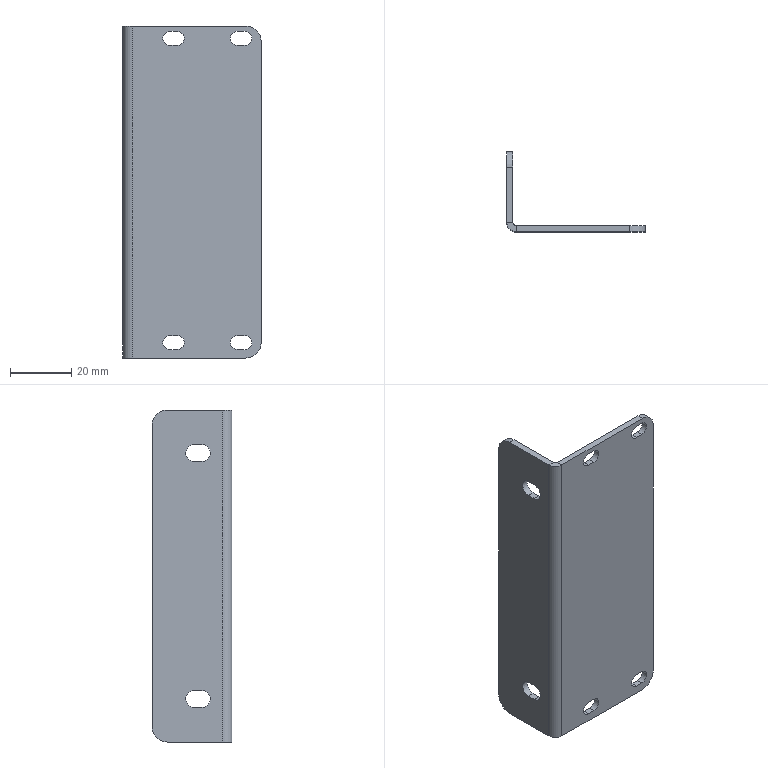Part | SolidWorks | features HoleWzd 2, Fillet 1, FlatPattern 1, SMBaseFlange 1, SheetMetal 1 | 1 solid | 42 faces | box 45 x 26 x 108 mm | volume 14308 mm3 | plane 24 | cylinder 18 | commonest cylinder face diameters 4.5 x8 5.5 x4 10 x4 2 x1 6 x1
STEP:
#1=CARTESIAN_POINT('',(0.,-23.,108.));
#2=VERTEX_POINT('',#1);
#3=CARTESIAN_POINT('',(2.,-23.,108.));
#4=VERTEX_POINT('',#3);
#5=CARTESIAN_POINT('',(0.,-23.,108.));
#6=DIRECTION('',(1.,0.,0.));
#7=VECTOR('',#6,1000.);
#8=LINE('',#5,#7);
#9=EDGE_CURVE('',#2,#4,#8,.T.);
#10=ORIENTED_EDGE('',*,*,#9,.F.);
#11=CARTESIAN_POINT('',(3.,-26.,108.));
#12=VERTEX_POINT('',#11);
#13=CARTESIAN_POINT('',(3.,-23.,108.));
#14=DIRECTION('',(0.,0.,1.));
#15=DIRECTION('',(-1.,0.,0.));
#16=AXIS2_PLACEMENT_3D('',#13,#14,#15);
#17=CIRCLE('',#16,3.);
#18=EDGE_CURVE('',#2,#12,#17,.T.);
#19=ORIENTED_EDGE('',*,*,#18,.T.);
#20=CARTESIAN_POINT('',(3.,-24.,108.));
#21=VERTEX_POINT('',#20);
#22=CARTESIAN_POINT('',(3.,-24.,108.));
#23=DIRECTION('',(0.,-1.,0.));
#24=VECTOR('',#23,1000.);
#25=LINE('',#22,#24);
#26=EDGE_CURVE('',#21,#12,#25,.T.);
#27=ORIENTED_EDGE('',*,*,#26,.F.);
#28=CARTESIAN_POINT('',(3.,-23.,108.));
#29=DIRECTION('',(0.,0.,1.));
#30=DIRECTION('',(1.,0.,0.));
#31=AXIS2_PLACEMENT_3D('',#28,#29,#30);
#32=CIRCLE('',#31,1.);
#33=EDGE_CURVE('',#4,#21,#32,.T.);
#34=ORIENTED_EDGE('',*,*,#33,.F.);
#35=EDGE_LOOP('',(#10,#19,#27,#34));
#36=FACE_OUTER_BOUND('',#35,.T.);
#37=CARTESIAN_POINT('',(0.,-23.,108.));
#38=DIRECTION('',(0.,0.,1.));
#39=DIRECTION('',(1.,0.,0.));
#40=AXIS2_PLACEMENT_3D('',#37,#38,#39);
#41=PLANE('',#40);
#42=ADVANCED_FACE('',(#36),#41,.T.);
#43=CARTESIAN_POINT('',(2.,-5.,108.));
#44=VERTEX_POINT('',#43);
#45=CARTESIAN_POINT('',(2.,0.,108.));
#46=DIRECTION('',(0.,-1.,0.));
#47=VECTOR('',#46,1000.);
#48=LINE('',#45,#47);
#49=EDGE_CURVE('',#44,#4,#48,.T.);
#50=ORIENTED_EDGE('',*,*,#49,.F.);
#51=CARTESIAN_POINT('',(0.,-5.,108.));
#52=VERTEX_POINT('',#51);
#53=CARTESIAN_POINT('',(3.,-5.,108.));
#54=DIRECTION('',(-1.,0.,0.));
#55=VECTOR('',#54,1000.);
#56=LINE('',#53,#55);
#57=EDGE_CURVE('',#44,#52,#56,.T.);
#58=ORIENTED_EDGE('',*,*,#57,.T.);
#59=CARTESIAN_POINT('',(0.,0.,108.));
#60=DIRECTION('',(0.,-1.,0.));
#61=VECTOR('',#60,1000.);
#62=LINE('',#59,#61);
#63=EDGE_CURVE('',#52,#2,#62,.T.);
#64=ORIENTED_EDGE('',*,*,#63,.T.);
#65=ORIENTED_EDGE('',*,*,#9,.T.);
#66=EDGE_LOOP('',(#50,#58,#64,#65));
#67=FACE_OUTER_BOUND('',#66,.T.);
#68=CARTESIAN_POINT('',(3.,-24.,108.));
#69=DIRECTION('',(0.,0.,1.));
#70=DIRECTION('',(1.,0.,0.));
#71=AXIS2_PLACEMENT_3D('',#68,#69,#70);
#72=PLANE('',#71);
#73=ADVANCED_FACE('',(#67),#72,.T.);
#74=CARTESIAN_POINT('',(3.,-26.,0.));
#75=VERTEX_POINT('',#74);
#76=CARTESIAN_POINT('',(3.,-24.,0.));
#77=VERTEX_POINT('',#76);
#78=CARTESIAN_POINT('',(3.,-26.,0.));
#79=DIRECTION('',(0.,1.,0.));
#80=VECTOR('',#79,1000.);
#81=LINE('',#78,#80);
#82=EDGE_CURVE('',#75,#77,#81,.T.);
#83=ORIENTED_EDGE('',*,*,#82,.F.);
#84=CARTESIAN_POINT('',(0.,-23.,0.));
#85=VERTEX_POINT('',#84);
#86=CARTESIAN_POINT('',(3.,-23.,0.));
#87=DIRECTION('',(0.,0.,1.));
#88=DIRECTION('',(-1.,0.,0.));
#89=AXIS2_PLACEMENT_3D('',#86,#87,#88);
#90=CIRCLE('',#89,3.);
#91=EDGE_CURVE('',#85,#75,#90,.T.);
#92=ORIENTED_EDGE('',*,*,#91,.F.);
#93=CARTESIAN_POINT('',(2.,-23.,0.));
#94=VERTEX_POINT('',#93);
#95=CARTESIAN_POINT('',(2.,-23.,0.));
#96=DIRECTION('',(-1.,0.,0.));
#97=VECTOR('',#96,1000.);
#98=LINE('',#95,#97);
#99=EDGE_CURVE('',#94,#85,#98,.T.);
#100=ORIENTED_EDGE('',*,*,#99,.F.);
#101=CARTESIAN_POINT('',(3.,-23.,0.));
#102=DIRECTION('',(0.,0.,1.));
#103=DIRECTION('',(1.,0.,0.));
#104=AXIS2_PLACEMENT_3D('',#101,#102,#103);
#105=CIRCLE('',#104,1.);
#106=EDGE_CURVE('',#94,#77,#105,.T.);
#107=ORIENTED_EDGE('',*,*,#106,.T.);
#108=EDGE_LOOP('',(#83,#92,#100,#107));
#109=FACE_OUTER_BOUND('',#108,.T.);
#110=CARTESIAN_POINT('',(3.,-26.,0.));
#111=DIRECTION('',(0.,0.,-1.));
#112=DIRECTION('',(-1.,0.,0.));
#113=AXIS2_PLACEMENT_3D('',#110,#111,#112);
#114=PLANE('',#113);
#115=ADVANCED_FACE('',(#109),#114,.T.);
#116=CARTESIAN_POINT('',(40.,-24.,0.));
#117=VERTEX_POINT('',#116);
#118=CARTESIAN_POINT('',(0.,-24.,0.));
#119=DIRECTION('',(1.,0.,0.));
#120=VECTOR('',#119,1000.);
#121=LINE('',#118,#120);
#122=EDGE_CURVE('',#77,#117,#121,.T.);
#123=ORIENTED_EDGE('',*,*,#122,.T.);
#124=CARTESIAN_POINT('',(40.,-26.,0.));
#125=VERTEX_POINT('',#124);
#126=CARTESIAN_POINT('',(40.,-23.,0.));
#127=DIRECTION('',(0.,-1.,0.));
#128=VECTOR('',#127,1000.);
#129=LINE('',#126,#128);
#130=EDGE_CURVE('',#117,#125,#129,.T.);
#131=ORIENTED_EDGE('',*,*,#130,.T.);
#132=CARTESIAN_POINT('',(0.,-26.,0.));
#133=DIRECTION('',(1.,0.,0.));
#134=VECTOR('',#133,1000.);
#135=LINE('',#132,#134);
#136=EDGE_CURVE('',#75,#125,#135,.T.);
#137=ORIENTED_EDGE('',*,*,#136,.F.);
#138=ORIENTED_EDGE('',*,*,#82,.T.);
#139=EDGE_LOOP('',(#123,#131,#137,#138));
#140=FACE_OUTER_BOUND('',#139,.T.);
#141=CARTESIAN_POINT('',(2.,-23.,0.));
#142=DIRECTION('',(0.,0.,-1.));
#143=DIRECTION('',(-1.,0.,0.));
#144=AXIS2_PLACEMENT_3D('',#141,#142,#143);
#145=PLANE('',#144);
#146=ADVANCED_FACE('',(#140),#145,.T.);
#147=CARTESIAN_POINT('',(37.25,-26.,7.25));
#148=VERTEX_POINT('',#147);
#149=CARTESIAN_POINT('',(39.75,-26.,7.25));
#150=VERTEX_POINT('',#149);
#151=CARTESIAN_POINT('',(0.,-26.,7.25));
#152=DIRECTION('',(1.,0.,0.));
#153=VECTOR('',#152,1000.);
#154=LINE('',#151,#153);
#155=EDGE_CURVE('',#148,#150,#154,.T.);
#156=ORIENTED_EDGE('',*,*,#155,.T.);
#157=CARTESIAN_POINT('',(39.75,-26.,2.75));
#158=VERTEX_POINT('',#157);
#159=CARTESIAN_POINT('',(39.75,-26.,5.));
#160=DIRECTION('',(0.,1.,0.));
#161=DIRECTION('',(0.,0.,1.));
#162=AXIS2_PLACEMENT_3D('',#159,#160,#161);
#163=CIRCLE('',#162,2.25);
#164=EDGE_CURVE('',#150,#158,#163,.T.);
#165=ORIENTED_EDGE('',*,*,#164,.T.);
#166=CARTESIAN_POINT('',(37.25,-26.,2.75));
#167=VERTEX_POINT('',#166);
#168=CARTESIAN_POINT('',(0.,-26.,2.75));
#169=DIRECTION('',(-1.,0.,0.));
#170=VECTOR('',#169,1000.);
#171=LINE('',#168,#170);
#172=EDGE_CURVE('',#158,#167,#171,.T.);
#173=ORIENTED_EDGE('',*,*,#172,.T.);
#174=CARTESIAN_POINT('',(37.25,-26.,5.));
#175=DIRECTION('',(0.,1.,0.));
#176=DIRECTION('',(0.,0.,1.));
#177=AXIS2_PLACEMENT_3D('',#174,#175,#176);
#178=CIRCLE('',#177,2.25);
#179=EDGE_CURVE('',#167,#148,#178,.T.);
#180=ORIENTED_EDGE('',*,*,#179,.T.);
#181=EDGE_LOOP('',(#156,#165,#173,#180));
#182=FACE_BOUND('',#181,.T.);
#183=CARTESIAN_POINT('',(17.75,-26.,7.25));
#184=VERTEX_POINT('',#183);
#185=CARTESIAN_POINT('',(17.75,-26.,2.75));
#186=VERTEX_POINT('',#185);
#187=CARTESIAN_POINT('',(17.75,-26.,5.));
#188=DIRECTION('',(0.,1.,0.));
#189=DIRECTION('',(0.,0.,1.));
#190=AXIS2_PLACEMENT_3D('',#187,#188,#189);
#191=CIRCLE('',#190,2.25);
#192=EDGE_CURVE('',#184,#186,#191,.T.);
#193=ORIENTED_EDGE('',*,*,#192,.T.);
#194=CARTESIAN_POINT('',(15.25,-26.,2.75));
#195=VERTEX_POINT('',#194);
#196=CARTESIAN_POINT('',(0.,-26.,2.75));
#197=DIRECTION('',(-1.,0.,0.));
#198=VECTOR('',#197,1000.);
#199=LINE('',#196,#198);
#200=EDGE_CURVE('',#186,#195,#199,.T.);
#201=ORIENTED_EDGE('',*,*,#200,.T.);
#202=CARTESIAN_POINT('',(15.25,-26.,7.25));
#203=VERTEX_POINT('',#202);
#204=CARTESIAN_POINT('',(15.25,-26.,5.));
#205=DIRECTION('',(0.,1.,0.));
#206=DIRECTION('',(0.,0.,1.));
#207=AXIS2_PLACEMENT_3D('',#204,#205,#206);
#208=CIRCLE('',#207,2.25);
#209=EDGE_CURVE('',#195,#203,#208,.T.);
#210=ORIENTED_EDGE('',*,*,#209,.T.);
#211=CARTESIAN_POINT('',(0.,-26.,7.25));
#212=DIRECTION('',(1.,0.,0.));
#213=VECTOR('',#212,1000.);
#214=LINE('',#211,#213);
#215=EDGE_CURVE('',#203,#184,#214,.T.);
#216=ORIENTED_EDGE('',*,*,#215,.T.);
#217=EDGE_LOOP('',(#193,#201,#210,#216));
#218=FACE_BOUND('',#217,.T.);
#219=CARTESIAN_POINT('',(39.75,-26.,101.75));
#220=VERTEX_POINT('',#219);
#221=CARTESIAN_POINT('',(37.25,-26.,101.75));
#222=VERTEX_POINT('',#221);
#223=CARTESIAN_POINT('',(0.,-26.,101.75));
#224=DIRECTION('',(-1.,0.,0.));
#225=VECTOR('',#224,1000.);
#226=LINE('',#223,#225);
#227=EDGE_CURVE('',#220,#222,#226,.T.);
#228=ORIENTED_EDGE('',*,*,#227,.T.);
#229=CARTESIAN_POINT('',(37.25,-26.,106.25));
#230=VERTEX_POINT('',#229);
#231=CARTESIAN_POINT('',(37.25,-26.,104.));
#232=DIRECTION('',(0.,1.,0.));
#233=DIRECTION('',(0.,0.,1.));
#234=AXIS2_PLACEMENT_3D('',#231,#232,#233);
#235=CIRCLE('',#234,2.25);
#236=EDGE_CURVE('',#222,#230,#235,.T.);
#237=ORIENTED_EDGE('',*,*,#236,.T.);
#238=CARTESIAN_POINT('',(39.75,-26.,106.25));
#239=VERTEX_POINT('',#238);
#240=CARTESIAN_POINT('',(0.,-26.,106.25));
#241=DIRECTION('',(1.,0.,0.));
#242=VECTOR('',#241,1000.);
#243=LINE('',#240,#242);
#244=EDGE_CURVE('',#230,#239,#243,.T.);
#245=ORIENTED_EDGE('',*,*,#244,.T.);
#246=CARTESIAN_POINT('',(39.75,-26.,104.));
#247=DIRECTION('',(0.,1.,0.));
#248=DIRECTION('',(0.,0.,1.));
#249=AXIS2_PLACEMENT_3D('',#246,#247,#248);
#250=CIRCLE('',#249,2.25);
#251=EDGE_CURVE('',#239,#220,#250,.T.);
#252=ORIENTED_EDGE('',*,*,#251,.T.);
#253=EDGE_LOOP('',(#228,#237,#245,#252));
#254=FACE_BOUND('',#253,.T.);
#255=CARTESIAN_POINT('',(17.75,-26.,106.25));
#256=VERTEX_POINT('',#255);
#257=CARTESIAN_POINT('',(17.75,-26.,101.75));
#258=VERTEX_POINT('',#257);
#259=CARTESIAN_POINT('',(17.75,-26.,104.));
#260=DIRECTION('',(0.,1.,0.));
#261=DIRECTION('',(0.,0.,1.));
#262=AXIS2_PLACEMENT_3D('',#259,#260,#261);
#263=CIRCLE('',#262,2.25);
#264=EDGE_CURVE('',#256,#258,#263,.T.);
#265=ORIENTED_EDGE('',*,*,#264,.T.);
#266=CARTESIAN_POINT('',(15.25,-26.,101.75));
#267=VERTEX_POINT('',#266);
#268=CARTESIAN_POINT('',(0.,-26.,101.75));
#269=DIRECTION('',(-1.,0.,0.));
#270=VECTOR('',#269,1000.);
#271=LINE('',#268,#270);
#272=EDGE_CURVE('',#258,#267,#271,.T.);
#273=ORIENTED_EDGE('',*,*,#272,.T.);
#274=CARTESIAN_POINT('',(15.25,-26.,106.25));
#275=VERTEX_POINT('',#274);
#276=CARTESIAN_POINT('',(15.25,-26.,104.));
#277=DIRECTION('',(0.,1.,0.));
#278=DIRECTION('',(0.,0.,1.));
#279=AXIS2_PLACEMENT_3D('',#276,#277,#278);
#280=CIRCLE('',#279,2.25);
#281=EDGE_CURVE('',#267,#275,#280,.T.);
#282=ORIENTED_EDGE('',*,*,#281,.T.);
#283=CARTESIAN_POINT('',(0.,-26.,106.25));
#284=DIRECTION('',(1.,0.,0.));
#285=VECTOR('',#284,1000.);
#286=LINE('',#283,#285);
#287=EDGE_CURVE('',#275,#256,#286,.T.);
#288=ORIENTED_EDGE('',*,*,#287,.T.);
#289=EDGE_LOOP('',(#265,#273,#282,#288));
#290=FACE_BOUND('',#289,.T.);
#291=ORIENTED_EDGE('',*,*,#136,.T.);
#292=CARTESIAN_POINT('',(45.,-26.,5.));
#293=VERTEX_POINT('',#292);
#294=CARTESIAN_POINT('',(40.,-26.,5.));
#295=DIRECTION('',(0.,-1.,0.));
#296=DIRECTION('',(0.,0.,1.));
#297=AXIS2_PLACEMENT_3D('',#294,#295,#296);
#298=CIRCLE('',#297,5.);
#299=EDGE_CURVE('',#125,#293,#298,.T.);
#300=ORIENTED_EDGE('',*,*,#299,.T.);
#301=CARTESIAN_POINT('',(45.,-26.,103.));
#302=VERTEX_POINT('',#301);
#303=CARTESIAN_POINT('',(45.,-26.,108.));
#304=DIRECTION('',(0.,0.,-1.));
#305=VECTOR('',#304,1000.);
#306=LINE('',#303,#305);
#307=EDGE_CURVE('',#302,#293,#306,.T.);
#308=ORIENTED_EDGE('',*,*,#307,.F.);
#309=CARTESIAN_POINT('',(40.,-26.,108.));
#310=VERTEX_POINT('',#309);
#311=CARTESIAN_POINT('',(40.,-26.,103.));
#312=DIRECTION('',(0.,-1.,0.));
#313=DIRECTION('',(0.,0.,1.));
#314=AXIS2_PLACEMENT_3D('',#311,#312,#313);
#315=CIRCLE('',#314,5.);
#316=EDGE_CURVE('',#302,#310,#315,.T.);
#317=ORIENTED_EDGE('',*,*,#316,.T.);
#318=CARTESIAN_POINT('',(0.,-26.,108.));
#319=DIRECTION('',(1.,0.,0.));
#320=VECTOR('',#319,1000.);
#321=LINE('',#318,#320);
#322=EDGE_CURVE('',#12,#310,#321,.T.);
#323=ORIENTED_EDGE('',*,*,#322,.F.);
#324=CARTESIAN_POINT('',(3.,-26.,108.));
#325=DIRECTION('',(0.,0.,-1.));
#326=VECTOR('',#325,1000.);
#327=LINE('',#324,#326);
#328=EDGE_CURVE('',#12,#75,#327,.T.);
#329=ORIENTED_EDGE('',*,*,#328,.T.);
#330=EDGE_LOOP('',(#291,#300,#308,#317,#323,#329));
#331=FACE_OUTER_BOUND('',#330,.T.);
#332=CARTESIAN_POINT('',(0.,-26.,108.));
#333=DIRECTION('',(0.,1.,0.));
#334=DIRECTION('',(0.,0.,1.));
#335=AXIS2_PLACEMENT_3D('',#332,#333,#334);
#336=PLANE('',#335);
#337=ADVANCED_FACE('',(#182,#218,#254,#290,#331),#336,.F.);
#338=ORIENTED_EDGE('',*,*,#307,.T.);
#339=CARTESIAN_POINT('',(45.,-24.,5.));
#340=VERTEX_POINT('',#339);
#341=CARTESIAN_POINT('',(45.,-24.,5.));
#342=DIRECTION('',(0.,1.,0.));
#343=VECTOR('',#342,1000.);
#344=LINE('',#341,#343);
#345=EDGE_CURVE('',#293,#340,#344,.T.);
#346=ORIENTED_EDGE('',*,*,#345,.T.);
#347=CARTESIAN_POINT('',(45.,-24.,103.));
#348=VERTEX_POINT('',#347);
#349=CARTESIAN_POINT('',(45.,-24.,108.));
#350=DIRECTION('',(0.,0.,-1.));
#351=VECTOR('',#350,1000.);
#352=LINE('',#349,#351);
#353=EDGE_CURVE('',#348,#340,#352,.T.);
#354=ORIENTED_EDGE('',*,*,#353,.F.);
#355=CARTESIAN_POINT('',(45.,-24.,103.));
#356=DIRECTION('',(0.,-1.,0.));
#357=VECTOR('',#356,1000.);
#358=LINE('',#355,#357);
#359=EDGE_CURVE('',#348,#302,#358,.T.);
#360=ORIENTED_EDGE('',*,*,#359,.T.);
#361=EDGE_LOOP('',(#338,#346,#354,#360));
#362=FACE_OUTER_BOUND('',#361,.T.);
#363=CARTESIAN_POINT('',(45.,-24.,108.));
#364=DIRECTION('',(1.,0.,0.));
#365=DIRECTION('',(0.,0.,-1.));
#366=AXIS2_PLACEMENT_3D('',#363,#364,#365);
#367=PLANE('',#366);
#368=ADVANCED_FACE('',(#362),#367,.T.);
#369=CARTESIAN_POINT('',(37.25,-24.,7.25));
#370=VERTEX_POINT('',#369);
#371=CARTESIAN_POINT('',(39.75,-24.,7.25));
#372=VERTEX_POINT('',#371);
#373=CARTESIAN_POINT('',(37.25,-24.,7.25));
#374=DIRECTION('',(1.,0.,0.));
#375=VECTOR('',#374,1000.);
#376=LINE('',#373,#375);
#377=EDGE_CURVE('',#370,#372,#376,.T.);
#378=ORIENTED_EDGE('',*,*,#377,.F.);
#379=CARTESIAN_POINT('',(37.25,-24.,2.75));
#380=VERTEX_POINT('',#379);
#381=CARTESIAN_POINT('',(37.25,-24.,5.));
#382=DIRECTION('',(0.,1.,0.));
#383=DIRECTION('',(0.,0.,1.));
#384=AXIS2_PLACEMENT_3D('',#381,#382,#383);
#385=CIRCLE('',#384,2.25);
#386=EDGE_CURVE('',#380,#370,#385,.T.);
#387=ORIENTED_EDGE('',*,*,#386,.F.);
#388=CARTESIAN_POINT('',(39.75,-24.,2.75));
#389=VERTEX_POINT('',#388);
#390=CARTESIAN_POINT('',(37.25,-24.,2.75));
#391=DIRECTION('',(1.,0.,0.));
#392=VECTOR('',#391,1000.);
#393=LINE('',#390,#392);
#394=EDGE_CURVE('',#380,#389,#393,.T.);
#395=ORIENTED_EDGE('',*,*,#394,.T.);
#396=CARTESIAN_POINT('',(39.75,-24.,5.));
#397=DIRECTION('',(0.,1.,0.));
#398=DIRECTION('',(0.,0.,1.));
#399=AXIS2_PLACEMENT_3D('',#396,#397,#398);
#400=CIRCLE('',#399,2.25);
#401=EDGE_CURVE('',#372,#389,#400,.T.);
#402=ORIENTED_EDGE('',*,*,#401,.F.);
#403=EDGE_LOOP('',(#378,#387,#395,#402));
#404=FACE_BOUND('',#403,.T.);
#405=CARTESIAN_POINT('',(15.25,-24.,7.25));
#406=VERTEX_POINT('',#405);
#407=CARTESIAN_POINT('',(17.75,-24.,7.25));
#408=VERTEX_POINT('',#407);
#409=CARTESIAN_POINT('',(15.25,-24.,7.25));
#410=DIRECTION('',(1.,0.,0.));
#411=VECTOR('',#410,1000.);
#412=LINE('',#409,#411);
#413=EDGE_CURVE('',#406,#408,#412,.T.);
#414=ORIENTED_EDGE('',*,*,#413,.F.);
#415=CARTESIAN_POINT('',(15.25,-24.,2.75));
#416=VERTEX_POINT('',#415);
#417=CARTESIAN_POINT('',(15.25,-24.,5.));
#418=DIRECTION('',(0.,1.,0.));
#419=DIRECTION('',(0.,0.,1.));
#420=AXIS2_PLACEMENT_3D('',#417,#418,#419);
#421=CIRCLE('',#420,2.25);
#422=EDGE_CURVE('',#416,#406,#421,.T.);
#423=ORIENTED_EDGE('',*,*,#422,.F.);
#424=CARTESIAN_POINT('',(17.75,-24.,2.75));
#425=VERTEX_POINT('',#424);
#426=CARTESIAN_POINT('',(15.25,-24.,2.75));
#427=DIRECTION('',(1.,0.,0.));
#428=VECTOR('',#427,1000.);
#429=LINE('',#426,#428);
#430=EDGE_CURVE('',#416,#425,#429,.T.);
#431=ORIENTED_EDGE('',*,*,#430,.T.);
#432=CARTESIAN_POINT('',(17.75,-24.,5.));
#433=DIRECTION('',(0.,1.,0.));
#434=DIRECTION('',(0.,0.,1.));
#435=AXIS2_PLACEMENT_3D('',#432,#433,#434);
#436=CIRCLE('',#435,2.25);
#437=EDGE_CURVE('',#408,#425,#436,.T.);
#438=ORIENTED_EDGE('',*,*,#437,.F.);
#439=EDGE_LOOP('',(#414,#423,#431,#438));
#440=FACE_BOUND('',#439,.T.);
#441=CARTESIAN_POINT('',(39.75,-24.,106.25));
#442=VERTEX_POINT('',#441);
#443=CARTESIAN_POINT('',(39.75,-24.,101.75));
#444=VERTEX_POINT('',#443);
#445=CARTESIAN_POINT('',(39.75,-24.,104.));
#446=DIRECTION('',(0.,1.,0.));
#447=DIRECTION('',(0.,0.,1.));
#448=AXIS2_PLACEMENT_3D('',#445,#446,#447);
#449=CIRCLE('',#448,2.25);
#450=EDGE_CURVE('',#442,#444,#449,.T.);
#451=ORIENTED_EDGE('',*,*,#450,.F.);
#452=CARTESIAN_POINT('',(37.25,-24.,106.25));
#453=VERTEX_POINT('',#452);
#454=CARTESIAN_POINT('',(37.25,-24.,106.25));
#455=DIRECTION('',(1.,0.,0.));
#456=VECTOR('',#455,1000.);
#457=LINE('',#454,#456);
#458=EDGE_CURVE('',#453,#442,#457,.T.);
#459=ORIENTED_EDGE('',*,*,#458,.F.);
#460=CARTESIAN_POINT('',(37.25,-24.,101.75));
#461=VERTEX_POINT('',#460);
#462=CARTESIAN_POINT('',(37.25,-24.,104.));
#463=DIRECTION('',(0.,1.,0.));
#464=DIRECTION('',(0.,0.,1.));
#465=AXIS2_PLACEMENT_3D('',#462,#463,#464);
#466=CIRCLE('',#465,2.25);
#467=EDGE_CURVE('',#461,#453,#466,.T.);
#468=ORIENTED_EDGE('',*,*,#467,.F.);
#469=CARTESIAN_POINT('',(37.25,-24.,101.75));
#470=DIRECTION('',(1.,0.,0.));
#471=VECTOR('',#470,1000.);
#472=LINE('',#469,#471);
#473=EDGE_CURVE('',#461,#444,#472,.T.);
#474=ORIENTED_EDGE('',*,*,#473,.T.);
#475=EDGE_LOOP('',(#451,#459,#468,#474));
#476=FACE_BOUND('',#475,.T.);
#477=CARTESIAN_POINT('',(15.25,-24.,106.25));
#478=VERTEX_POINT('',#477);
#479=CARTESIAN_POINT('',(17.75,-24.,106.25));
#480=VERTEX_POINT('',#479);
#481=CARTESIAN_POINT('',(15.25,-24.,106.25));
#482=DIRECTION('',(1.,0.,0.));
#483=VECTOR('',#482,1000.);
#484=LINE('',#481,#483);
#485=EDGE_CURVE('',#478,#480,#484,.T.);
#486=ORIENTED_EDGE('',*,*,#485,.F.);
#487=CARTESIAN_POINT('',(15.25,-24.,101.75));
#488=VERTEX_POINT('',#487);
#489=CARTESIAN_POINT('',(15.25,-24.,104.));
#490=DIRECTION('',(0.,1.,0.));
#491=DIRECTION('',(0.,0.,1.));
#492=AXIS2_PLACEMENT_3D('',#489,#490,#491);
#493=CIRCLE('',#492,2.25);
#494=EDGE_CURVE('',#488,#478,#493,.T.);
#495=ORIENTED_EDGE('',*,*,#494,.F.);
#496=CARTESIAN_POINT('',(17.75,-24.,101.75));
#497=VERTEX_POINT('',#496);
#498=CARTESIAN_POINT('',(15.25,-24.,101.75));
#499=DIRECTION('',(1.,0.,0.));
#500=VECTOR('',#499,1000.);
#501=LINE('',#498,#500);
#502=EDGE_CURVE('',#488,#497,#501,.T.);
#503=ORIENTED_EDGE('',*,*,#502,.T.);
#504=CARTESIAN_POINT('',(17.75,-24.,104.));
#505=DIRECTION('',(0.,1.,0.));
#506=DIRECTION('',(0.,0.,1.));
#507=AXIS2_PLACEMENT_3D('',#504,#505,#506);
#508=CIRCLE('',#507,2.25);
#509=EDGE_CURVE('',#480,#497,#508,.T.);
#510=ORIENTED_EDGE('',*,*,#509,.F.);
#511=EDGE_LOOP('',(#486,#495,#503,#510));
#512=FACE_BOUND('',#511,.T.);
#513=ORIENTED_EDGE('',*,*,#353,.T.);
#514=CARTESIAN_POINT('',(40.,-24.,5.));
#515=DIRECTION('',(0.,1.,0.));
#516=DIRECTION('',(0.,0.,1.));
#517=AXIS2_PLACEMENT_3D('',#514,#515,#516);
#518=CIRCLE('',#517,5.);
#519=EDGE_CURVE('',#340,#117,#518,.T.);
#520=ORIENTED_EDGE('',*,*,#519,.T.);
#521=ORIENTED_EDGE('',*,*,#122,.F.);
#522=CARTESIAN_POINT('',(3.,-24.,108.));
#523=DIRECTION('',(0.,0.,-1.));
#524=VECTOR('',#523,1000.);
#525=LINE('',#522,#524);
#526=EDGE_CURVE('',#21,#77,#525,.T.);
#527=ORIENTED_EDGE('',*,*,#526,.F.);
#528=CARTESIAN_POINT('',(40.,-24.,108.));
#529=VERTEX_POINT('',#528);
#530=CARTESIAN_POINT('',(0.,-24.,108.));
#531=DIRECTION('',(1.,0.,0.));
#532=VECTOR('',#531,1000.);
#533=LINE('',#530,#532);
#534=EDGE_CURVE('',#21,#529,#533,.T.);
#535=ORIENTED_EDGE('',*,*,#534,.T.);
#536=CARTESIAN_POINT('',(40.,-24.,103.));
#537=DIRECTION('',(0.,1.,0.));
#538=DIRECTION('',(0.,0.,1.));
#539=AXIS2_PLACEMENT_3D('',#536,#537,#538);
#540=CIRCLE('',#539,5.);
#541=EDGE_CURVE('',#529,#348,#540,.T.);
#542=ORIENTED_EDGE('',*,*,#541,.T.);
#543=EDGE_LOOP('',(#513,#520,#521,#527,#535,#542));
#544=FACE_OUTER_BOUND('',#543,.T.);
#545=CARTESIAN_POINT('',(0.,-24.,108.));
#546=DIRECTION('',(0.,1.,0.));
#547=DIRECTION('',(0.,0.,1.));
#548=AXIS2_PLACEMENT_3D('',#545,#546,#547);
#549=PLANE('',#548);
#550=ADVANCED_FACE('',(#404,#440,#476,#512,#544),#549,.T.);
#551=ORIENTED_EDGE('',*,*,#106,.F.);
#552=CARTESIAN_POINT('',(2.,-23.,108.));
#553=DIRECTION('',(0.,0.,-1.));
#554=VECTOR('',#553,1000.);
#555=LINE('',#552,#554);
#556=EDGE_CURVE('',#4,#94,#555,.T.);
#557=ORIENTED_EDGE('',*,*,#556,.F.);
#558=ORIENTED_EDGE('',*,*,#33,.T.);
#559=ORIENTED_EDGE('',*,*,#526,.T.);
#560=EDGE_LOOP('',(#551,#557,#558,#559));
#561=FACE_OUTER_BOUND('',#560,.T.);
#562=CARTESIAN_POINT('',(3.,-23.,108.));
#563=DIRECTION('',(0.,0.,-1.));
#564=DIRECTION('',(-1.,0.,0.));
#565=AXIS2_PLACEMENT_3D('',#562,#563,#564);
#566=CYLINDRICAL_SURFACE('',#565,1.);
#567=ADVANCED_FACE('',(#561),#566,.F.);
#568=CARTESIAN_POINT('',(2.,-13.75,11.25));
#569=VERTEX_POINT('',#568);
#570=CARTESIAN_POINT('',(2.,-13.75,16.75));
#571=VERTEX_POINT('',#570);
#572=CARTESIAN_POINT('',(2.,-13.75,14.));
#573=DIRECTION('',(1.,0.,0.));
#574=DIRECTION('',(0.,0.,-1.));
#575=AXIS2_PLACEMENT_3D('',#572,#573,#574);
#576=CIRCLE('',#575,2.75);
#577=EDGE_CURVE('',#569,#571,#576,.T.);
#578=ORIENTED_EDGE('',*,*,#577,.F.);
#579=CARTESIAN_POINT('',(2.,-16.25,11.25));
#580=VERTEX_POINT('',#579);
#581=CARTESIAN_POINT('',(2.,-16.25,11.25));
#582=DIRECTION('',(0.,1.,0.));
#583=VECTOR('',#582,1000.);
#584=LINE('',#581,#583);
#585=EDGE_CURVE('',#580,#569,#584,.T.);
#586=ORIENTED_EDGE('',*,*,#585,.F.);
#587=CARTESIAN_POINT('',(2.,-16.25,16.75));
#588=VERTEX_POINT('',#587);
#589=CARTESIAN_POINT('',(2.,-16.25,14.));
#590=DIRECTION('',(1.,0.,0.));
#591=DIRECTION('',(0.,0.,-1.));
#592=AXIS2_PLACEMENT_3D('',#589,#590,#591);
#593=CIRCLE('',#592,2.75);
#594=EDGE_CURVE('',#588,#580,#593,.T.);
#595=ORIENTED_EDGE('',*,*,#594,.F.);
#596=CARTESIAN_POINT('',(2.,-16.25,16.75));
#597=DIRECTION('',(0.,1.,0.));
#598=VECTOR('',#597,1000.);
#599=LINE('',#596,#598);
#600=EDGE_CURVE('',#588,#571,#599,.T.);
#601=ORIENTED_EDGE('',*,*,#600,.T.);
#602=EDGE_LOOP('',(#578,#586,#595,#601));
#603=FACE_BOUND('',#602,.T.);
#604=CARTESIAN_POINT('',(2.,-13.75,91.25));
#605=VERTEX_POINT('',#604);
#606=CARTESIAN_POINT('',(2.,-13.75,96.75));
#607=VERTEX_POINT('',#606);
#608=CARTESIAN_POINT('',(2.,-13.75,94.));
#609=DIRECTION('',(1.,0.,0.));
#610=DIRECTION('',(0.,0.,-1.));
#611=AXIS2_PLACEMENT_3D('',#608,#609,#610);
#612=CIRCLE('',#611,2.75);
#613=EDGE_CURVE('',#605,#607,#612,.T.);
#614=ORIENTED_EDGE('',*,*,#613,.F.);
#615=CARTESIAN_POINT('',(2.,-16.25,91.25));
#616=VERTEX_POINT('',#615);
#617=CARTESIAN_POINT('',(2.,-16.25,91.25));
#618=DIRECTION('',(0.,1.,0.));
#619=VECTOR('',#618,1000.);
#620=LINE('',#617,#619);
#621=EDGE_CURVE('',#616,#605,#620,.T.);
#622=ORIENTED_EDGE('',*,*,#621,.F.);
#623=CARTESIAN_POINT('',(2.,-16.25,96.75));
#624=VERTEX_POINT('',#623);
#625=CARTESIAN_POINT('',(2.,-16.25,94.));
#626=DIRECTION('',(1.,0.,0.));
#627=DIRECTION('',(0.,0.,-1.));
#628=AXIS2_PLACEMENT_3D('',#625,#626,#627);
#629=CIRCLE('',#628,2.75);
#630=EDGE_CURVE('',#624,#616,#629,.T.);
#631=ORIENTED_EDGE('',*,*,#630,.F.);
#632=CARTESIAN_POINT('',(2.,-16.25,96.75));
#633=DIRECTION('',(0.,1.,0.));
#634=VECTOR('',#633,1000.);
#635=LINE('',#632,#634);
#636=EDGE_CURVE('',#624,#607,#635,.T.);
#637=ORIENTED_EDGE('',*,*,#636,.T.);
#638=EDGE_LOOP('',(#614,#622,#631,#637));
#639=FACE_BOUND('',#638,.T.);
#640=CARTESIAN_POINT('',(2.,0.,103.));
#641=VERTEX_POINT('',#640);
#642=CARTESIAN_POINT('',(2.,0.,5.));
#643=VERTEX_POINT('',#642);
#644=CARTESIAN_POINT('',(2.,0.,108.));
#645=DIRECTION('',(0.,0.,-1.));
#646=VECTOR('',#645,1000.);
#647=LINE('',#644,#646);
#648=EDGE_CURVE('',#641,#643,#647,.T.);
#649=ORIENTED_EDGE('',*,*,#648,.F.);
#650=CARTESIAN_POINT('',(2.,-5.,103.));
#651=DIRECTION('',(1.,0.,0.));
#652=DIRECTION('',(0.,1.,0.));
#653=AXIS2_PLACEMENT_3D('',#650,#651,#652);
#654=CIRCLE('',#653,5.);
#655=EDGE_CURVE('',#641,#44,#654,.T.);
#656=ORIENTED_EDGE('',*,*,#655,.T.);
#657=ORIENTED_EDGE('',*,*,#49,.T.);
#658=ORIENTED_EDGE('',*,*,#556,.T.);
#659=CARTESIAN_POINT('',(2.,-5.,0.));
#660=VERTEX_POINT('',#659);
#661=CARTESIAN_POINT('',(2.,0.,0.));
#662=DIRECTION('',(0.,-1.,0.));
#663=VECTOR('',#662,1000.);
#664=LINE('',#661,#663);
#665=EDGE_CURVE('',#660,#94,#664,.T.);
#666=ORIENTED_EDGE('',*,*,#665,.F.);
#667=CARTESIAN_POINT('',(2.,-5.,5.));
#668=DIRECTION('',(1.,0.,0.));
#669=DIRECTION('',(0.,1.,0.));
#670=AXIS2_PLACEMENT_3D('',#667,#668,#669);
#671=CIRCLE('',#670,5.);
#672=EDGE_CURVE('',#660,#643,#671,.T.);
#673=ORIENTED_EDGE('',*,*,#672,.T.);
#674=EDGE_LOOP('',(#649,#656,#657,#658,#666,#673));
#675=FACE_OUTER_BOUND('',#674,.T.);
#676=CARTESIAN_POINT('',(2.,0.,108.));
#677=DIRECTION('',(1.,0.,0.));
#678=DIRECTION('',(0.,1.,0.));
#679=AXIS2_PLACEMENT_3D('',#676,#677,#678);
#680=PLANE('',#679);
#681=ADVANCED_FACE('',(#603,#639,#675),#680,.T.);
#682=CARTESIAN_POINT('',(0.,0.,103.));
#683=VERTEX_POINT('',#682);
#684=CARTESIAN_POINT('',(0.,0.,5.));
#685=VERTEX_POINT('',#684);
#686=CARTESIAN_POINT('',(0.,0.,108.));
#687=DIRECTION('',(0.,0.,-1.));
#688=VECTOR('',#687,1000.);
#689=LINE('',#686,#688);
#690=EDGE_CURVE('',#683,#685,#689,.T.);
#691=ORIENTED_EDGE('',*,*,#690,.F.);
#692=CARTESIAN_POINT('',(0.,0.,103.));
#693=DIRECTION('',(1.,0.,0.));
#694=VECTOR('',#693,1000.);
#695=LINE('',#692,#694);
#696=EDGE_CURVE('',#683,#641,#695,.T.);
#697=ORIENTED_EDGE('',*,*,#696,.T.);
#698=ORIENTED_EDGE('',*,*,#648,.T.);
#699=CARTESIAN_POINT('',(0.,0.,5.));
#700=DIRECTION('',(-1.,0.,0.));
#701=VECTOR('',#700,1000.);
#702=LINE('',#699,#701);
#703=EDGE_CURVE('',#643,#685,#702,.T.);
#704=ORIENTED_EDGE('',*,*,#703,.T.);
#705=EDGE_LOOP('',(#691,#697,#698,#704));
#706=FACE_OUTER_BOUND('',#705,.T.);
#707=CARTESIAN_POINT('',(0.,0.,108.));
#708=DIRECTION('',(0.,1.,0.));
#709=DIRECTION('',(-1.,0.,0.));
#710=AXIS2_PLACEMENT_3D('',#707,#708,#709);
#711=PLANE('',#710);
#712=ADVANCED_FACE('',(#706),#711,.T.);
#713=CARTESIAN_POINT('',(0.,-13.75,16.75));
#714=VERTEX_POINT('',#713);
#715=CARTESIAN_POINT('',(0.,-16.25,16.75));
#716=VERTEX_POINT('',#715);
#717=CARTESIAN_POINT('',(0.,0.,16.75));
#718=DIRECTION('',(0.,-1.,0.));
#719=VECTOR('',#718,1000.);
#720=LINE('',#717,#719);
#721=EDGE_CURVE('',#714,#716,#720,.T.);
#722=ORIENTED_EDGE('',*,*,#721,.T.);
#723=CARTESIAN_POINT('',(0.,-16.25,11.25));
#724=VERTEX_POINT('',#723);
#725=CARTESIAN_POINT('',(0.,-16.25,14.));
#726=DIRECTION('',(1.,0.,0.));
#727=DIRECTION('',(0.,1.,0.));
#728=AXIS2_PLACEMENT_3D('',#725,#726,#727);
#729=CIRCLE('',#728,2.75);
#730=EDGE_CURVE('',#716,#724,#729,.T.);
#731=ORIENTED_EDGE('',*,*,#730,.T.);
#732=CARTESIAN_POINT('',(0.,-13.75,11.25));
#733=VERTEX_POINT('',#732);
#734=CARTESIAN_POINT('',(0.,0.,11.25));
#735=DIRECTION('',(0.,1.,0.));
#736=VECTOR('',#735,1000.);
#737=LINE('',#734,#736);
#738=EDGE_CURVE('',#724,#733,#737,.T.);
#739=ORIENTED_EDGE('',*,*,#738,.T.);
#740=CARTESIAN_POINT('',(0.,-13.75,14.));
#741=DIRECTION('',(1.,0.,0.));
#742=DIRECTION('',(0.,1.,0.));
#743=AXIS2_PLACEMENT_3D('',#740,#741,#742);
#744=CIRCLE('',#743,2.75);
#745=EDGE_CURVE('',#733,#714,#744,.T.);
#746=ORIENTED_EDGE('',*,*,#745,.T.);
#747=EDGE_LOOP('',(#722,#731,#739,#746));
#748=FACE_BOUND('',#747,.T.);
#749=CARTESIAN_POINT('',(0.,-13.75,96.75));
#750=VERTEX_POINT('',#749);
#751=CARTESIAN_POINT('',(0.,-16.25,96.75));
#752=VERTEX_POINT('',#751);
#753=CARTESIAN_POINT('',(0.,0.,96.75));
#754=DIRECTION('',(0.,-1.,0.));
#755=VECTOR('',#754,1000.);
#756=LINE('',#753,#755);
#757=EDGE_CURVE('',#750,#752,#756,.T.);
#758=ORIENTED_EDGE('',*,*,#757,.T.);
#759=CARTESIAN_POINT('',(0.,-16.25,91.25));
#760=VERTEX_POINT('',#759);
#761=CARTESIAN_POINT('',(0.,-16.25,94.));
#762=DIRECTION('',(1.,0.,0.));
#763=DIRECTION('',(0.,1.,0.));
#764=AXIS2_PLACEMENT_3D('',#761,#762,#763);
#765=CIRCLE('',#764,2.75);
#766=EDGE_CURVE('',#752,#760,#765,.T.);
#767=ORIENTED_EDGE('',*,*,#766,.T.);
#768=CARTESIAN_POINT('',(0.,-13.75,91.25));
#769=VERTEX_POINT('',#768);
#770=CARTESIAN_POINT('',(0.,0.,91.25));
#771=DIRECTION('',(0.,1.,0.));
#772=VECTOR('',#771,1000.);
#773=LINE('',#770,#772);
#774=EDGE_CURVE('',#760,#769,#773,.T.);
#775=ORIENTED_EDGE('',*,*,#774,.T.);
#776=CARTESIAN_POINT('',(0.,-13.75,94.));
#777=DIRECTION('',(1.,0.,0.));
#778=DIRECTION('',(0.,1.,0.));
#779=AXIS2_PLACEMENT_3D('',#776,#777,#778);
#780=CIRCLE('',#779,2.75);
#781=EDGE_CURVE('',#769,#750,#780,.T.);
#782=ORIENTED_EDGE('',*,*,#781,.T.);
#783=EDGE_LOOP('',(#758,#767,#775,#782));
#784=FACE_BOUND('',#783,.T.);
#785=ORIENTED_EDGE('',*,*,#63,.F.);
#786=CARTESIAN_POINT('',(0.,-5.,103.));
#787=DIRECTION('',(-1.,0.,0.));
#788=DIRECTION('',(0.,1.,0.));
#789=AXIS2_PLACEMENT_3D('',#786,#787,#788);
#790=CIRCLE('',#789,5.);
#791=EDGE_CURVE('',#52,#683,#790,.T.);
#792=ORIENTED_EDGE('',*,*,#791,.T.);
#793=ORIENTED_EDGE('',*,*,#690,.T.);
#794=CARTESIAN_POINT('',(0.,-5.,0.));
#795=VERTEX_POINT('',#794);
#796=CARTESIAN_POINT('',(0.,-5.,5.));
#797=DIRECTION('',(-1.,0.,0.));
#798=DIRECTION('',(0.,1.,0.));
#799=AXIS2_PLACEMENT_3D('',#796,#797,#798);
#800=CIRCLE('',#799,5.);
#801=EDGE_CURVE('',#685,#795,#800,.T.);
#802=ORIENTED_EDGE('',*,*,#801,.T.);
#803=CARTESIAN_POINT('',(0.,0.,0.));
#804=DIRECTION('',(0.,-1.,0.));
#805=VECTOR('',#804,1000.);
#806=LINE('',#803,#805);
#807=EDGE_CURVE('',#795,#85,#806,.T.);
#808=ORIENTED_EDGE('',*,*,#807,.T.);
#809=CARTESIAN_POINT('',(0.,-23.,108.));
#810=DIRECTION('',(0.,0.,-1.));
#811=VECTOR('',#810,1000.);
#812=LINE('',#809,#811);
#813=EDGE_CURVE('',#2,#85,#812,.T.);
#814=ORIENTED_EDGE('',*,*,#813,.F.);
#815=EDGE_LOOP('',(#785,#792,#793,#802,#808,#814));
#816=FACE_OUTER_BOUND('',#815,.T.);
#817=CARTESIAN_POINT('',(0.,0.,108.));
#818=DIRECTION('',(1.,0.,0.));
#819=DIRECTION('',(0.,1.,0.));
#820=AXIS2_PLACEMENT_3D('',#817,#818,#819);
#821=PLANE('',#820);
#822=ADVANCED_FACE('',(#748,#784,#816),#821,.F.);
#823=ORIENTED_EDGE('',*,*,#91,.T.);
#824=ORIENTED_EDGE('',*,*,#328,.F.);
#825=ORIENTED_EDGE('',*,*,#18,.F.);
#826=ORIENTED_EDGE('',*,*,#813,.T.);
#827=EDGE_LOOP('',(#823,#824,#825,#826));
#828=FACE_OUTER_BOUND('',#827,.T.);
#829=CARTESIAN_POINT('',(3.,-23.,108.));
#830=DIRECTION('',(0.,0.,-1.));
#831=DIRECTION('',(-1.,0.,0.));
#832=AXIS2_PLACEMENT_3D('',#829,#830,#831);
#833=CYLINDRICAL_SURFACE('',#832,3.);
#834=ADVANCED_FACE('',(#828),#833,.T.);
#835=ORIENTED_EDGE('',*,*,#322,.T.);
#836=CARTESIAN_POINT('',(40.,-23.,108.));
#837=DIRECTION('',(0.,1.,0.));
#838=VECTOR('',#837,1000.);
#839=LINE('',#836,#838);
#840=EDGE_CURVE('',#310,#529,#839,.T.);
#841=ORIENTED_EDGE('',*,*,#840,.T.);
#842=ORIENTED_EDGE('',*,*,#534,.F.);
#843=ORIENTED_EDGE('',*,*,#26,.T.);
#844=EDGE_LOOP('',(#835,#841,#842,#843));
#845=FACE_OUTER_BOUND('',#844,.T.);
#846=CARTESIAN_POINT('',(3.,-23.,108.));
#847=DIRECTION('',(0.,0.,1.));
#848=DIRECTION('',(1.,0.,0.));
#849=AXIS2_PLACEMENT_3D('',#846,#847,#848);
#850=PLANE('',#849);
#851=ADVANCED_FACE('',(#845),#850,.T.);
#852=ORIENTED_EDGE('',*,*,#807,.F.);
#853=CARTESIAN_POINT('',(2.,-5.,0.));
#854=DIRECTION('',(1.,0.,0.));
#855=VECTOR('',#854,1000.);
#856=LINE('',#853,#855);
#857=EDGE_CURVE('',#795,#660,#856,.T.);
#858=ORIENTED_EDGE('',*,*,#857,.T.);
#859=ORIENTED_EDGE('',*,*,#665,.T.);
#860=ORIENTED_EDGE('',*,*,#99,.T.);
#861=EDGE_LOOP('',(#852,#858,#859,#860));
#862=FACE_OUTER_BOUND('',#861,.T.);
#863=CARTESIAN_POINT('',(3.,-23.,0.));
#864=DIRECTION('',(0.,0.,1.));
#865=DIRECTION('',(1.,0.,0.));
#866=AXIS2_PLACEMENT_3D('',#863,#864,#865);
#867=PLANE('',#866);
#868=ADVANCED_FACE('',(#862),#867,.F.);
#869=CARTESIAN_POINT('',(15.25,-24.,101.75));
#870=DIRECTION('',(0.,-1.,0.));
#871=VECTOR('',#870,1000.);
#872=LINE('',#869,#871);
#873=EDGE_CURVE('',#488,#267,#872,.T.);
#874=ORIENTED_EDGE('',*,*,#873,.F.);
#875=ORIENTED_EDGE('',*,*,#494,.T.);
#876=CARTESIAN_POINT('',(15.25,-24.,106.25));
#877=DIRECTION('',(0.,1.,0.));
#878=VECTOR('',#877,1000.);
#879=LINE('',#876,#878);
#880=EDGE_CURVE('',#275,#478,#879,.T.);
#881=ORIENTED_EDGE('',*,*,#880,.F.);
#882=ORIENTED_EDGE('',*,*,#281,.F.);
#883=EDGE_LOOP('',(#874,#875,#881,#882));
#884=FACE_OUTER_BOUND('',#883,.T.);
#885=CARTESIAN_POINT('',(15.25,-24.,104.));
#886=DIRECTION('',(0.,1.,0.));
#887=DIRECTION('',(0.,0.,1.));
#888=AXIS2_PLACEMENT_3D('',#885,#886,#887);
#889=CYLINDRICAL_SURFACE('',#888,2.25);
#890=ADVANCED_FACE('',(#884),#889,.F.);
#891=CARTESIAN_POINT('',(17.75,-24.,101.75));
#892=DIRECTION('',(0.,1.,0.));
#893=VECTOR('',#892,1000.);
#894=LINE('',#891,#893);
#895=EDGE_CURVE('',#258,#497,#894,.T.);
#896=ORIENTED_EDGE('',*,*,#895,.T.);
#897=ORIENTED_EDGE('',*,*,#502,.F.);
#898=ORIENTED_EDGE('',*,*,#873,.T.);
#899=ORIENTED_EDGE('',*,*,#272,.F.);
#900=EDGE_LOOP('',(#896,#897,#898,#899));
#901=FACE_OUTER_BOUND('',#900,.T.);
#902=CARTESIAN_POINT('',(15.25,-24.,101.75));
#903=DIRECTION('',(0.,0.,-1.));
#904=DIRECTION('',(-1.,0.,0.));
#905=AXIS2_PLACEMENT_3D('',#902,#903,#904);
#906=PLANE('',#905);
#907=ADVANCED_FACE('',(#901),#906,.F.);
#908=CARTESIAN_POINT('',(17.75,-24.,106.25));
#909=DIRECTION('',(0.,-1.,0.));
#910=VECTOR('',#909,1000.);
#911=LINE('',#908,#910);
#912=EDGE_CURVE('',#480,#256,#911,.T.);
#913=ORIENTED_EDGE('',*,*,#912,.F.);
#914=ORIENTED_EDGE('',*,*,#509,.T.);
#915=ORIENTED_EDGE('',*,*,#895,.F.);
#916=ORIENTED_EDGE('',*,*,#264,.F.);
#917=EDGE_LOOP('',(#913,#914,#915,#916));
#918=FACE_OUTER_BOUND('',#917,.T.);
#919=CARTESIAN_POINT('',(17.75,-24.,104.));
#920=DIRECTION('',(0.,1.,0.));
#921=DIRECTION('',(0.,0.,1.));
#922=AXIS2_PLACEMENT_3D('',#919,#920,#921);
#923=CYLINDRICAL_SURFACE('',#922,2.25);
#924=ADVANCED_FACE('',(#918),#923,.F.);
#925=ORIENTED_EDGE('',*,*,#880,.T.);
#926=ORIENTED_EDGE('',*,*,#485,.T.);
#927=ORIENTED_EDGE('',*,*,#912,.T.);
#928=ORIENTED_EDGE('',*,*,#287,.F.);
#929=EDGE_LOOP('',(#925,#926,#927,#928));
#930=FACE_OUTER_BOUND('',#929,.T.);
#931=CARTESIAN_POINT('',(15.25,-24.,106.25));
#932=DIRECTION('',(0.,0.,1.));
#933=DIRECTION('',(1.,0.,0.));
#934=AXIS2_PLACEMENT_3D('',#931,#932,#933);
#935=PLANE('',#934);
#936=ADVANCED_FACE('',(#930),#935,.F.);
#937=CARTESIAN_POINT('',(37.25,-24.,101.75));
#938=DIRECTION('',(0.,-1.,0.));
#939=VECTOR('',#938,1000.);
#940=LINE('',#937,#939);
#941=EDGE_CURVE('',#461,#222,#940,.T.);
#942=ORIENTED_EDGE('',*,*,#941,.F.);
#943=ORIENTED_EDGE('',*,*,#467,.T.);
#944=CARTESIAN_POINT('',(37.25,-24.,106.25));
#945=DIRECTION('',(0.,1.,0.));
#946=VECTOR('',#945,1000.);
#947=LINE('',#944,#946);
#948=EDGE_CURVE('',#230,#453,#947,.T.);
#949=ORIENTED_EDGE('',*,*,#948,.F.);
#950=ORIENTED_EDGE('',*,*,#236,.F.);
#951=EDGE_LOOP('',(#942,#943,#949,#950));
#952=FACE_OUTER_BOUND('',#951,.T.);
#953=CARTESIAN_POINT('',(37.25,-24.,104.));
#954=DIRECTION('',(0.,1.,0.));
#955=DIRECTION('',(0.,0.,1.));
#956=AXIS2_PLACEMENT_3D('',#953,#954,#955);
#957=CYLINDRICAL_SURFACE('',#956,2.25);
#958=ADVANCED_FACE('',(#952),#957,.F.);
#959=ORIENTED_EDGE('',*,*,#948,.T.);
#960=ORIENTED_EDGE('',*,*,#458,.T.);
#961=CARTESIAN_POINT('',(39.75,-24.,106.25));
#962=DIRECTION('',(0.,-1.,0.));
#963=VECTOR('',#962,1000.);
#964=LINE('',#961,#963);
#965=EDGE_CURVE('',#442,#239,#964,.T.);
#966=ORIENTED_EDGE('',*,*,#965,.T.);
#967=ORIENTED_EDGE('',*,*,#244,.F.);
#968=EDGE_LOOP('',(#959,#960,#966,#967));
#969=FACE_OUTER_BOUND('',#968,.T.);
#970=CARTESIAN_POINT('',(37.25,-24.,106.25));
#971=DIRECTION('',(0.,0.,1.));
#972=DIRECTION('',(1.,0.,0.));
#973=AXIS2_PLACEMENT_3D('',#970,#971,#972);
#974=PLANE('',#973);
#975=ADVANCED_FACE('',(#969),#974,.F.);
#976=ORIENTED_EDGE('',*,*,#965,.F.);
#977=ORIENTED_EDGE('',*,*,#450,.T.);
#978=CARTESIAN_POINT('',(39.75,-24.,101.75));
#979=DIRECTION('',(0.,1.,0.));
#980=VECTOR('',#979,1000.);
#981=LINE('',#978,#980);
#982=EDGE_CURVE('',#220,#444,#981,.T.);
#983=ORIENTED_EDGE('',*,*,#982,.F.);
#984=ORIENTED_EDGE('',*,*,#251,.F.);
#985=EDGE_LOOP('',(#976,#977,#983,#984));
#986=FACE_OUTER_BOUND('',#985,.T.);
#987=CARTESIAN_POINT('',(39.75,-24.,104.));
#988=DIRECTION('',(0.,1.,0.));
#989=DIRECTION('',(0.,0.,1.));
#990=AXIS2_PLACEMENT_3D('',#987,#988,#989);
#991=CYLINDRICAL_SURFACE('',#990,2.25);
#992=ADVANCED_FACE('',(#986),#991,.F.);
#993=ORIENTED_EDGE('',*,*,#982,.T.);
#994=ORIENTED_EDGE('',*,*,#473,.F.);
#995=ORIENTED_EDGE('',*,*,#941,.T.);
#996=ORIENTED_EDGE('',*,*,#227,.F.);
#997=EDGE_LOOP('',(#993,#994,#995,#996));
#998=FACE_OUTER_BOUND('',#997,.T.);
#999=CARTESIAN_POINT('',(37.25,-24.,101.75));
#1000=DIRECTION('',(0.,0.,-1.));
#1001=DIRECTION('',(-1.,0.,0.));
#1002=AXIS2_PLACEMENT_3D('',#999,#1000,#1001);
#1003=PLANE('',#1002);
#1004=ADVANCED_FACE('',(#998),#1003,.F.);
#1005=CARTESIAN_POINT('',(17.75,-24.,7.25));
#1006=DIRECTION('',(0.,-1.,0.));
#1007=VECTOR('',#1006,1000.);
#1008=LINE('',#1005,#1007);
#1009=EDGE_CURVE('',#408,#184,#1008,.T.);
#1010=ORIENTED_EDGE('',*,*,#1009,.F.);
#1011=ORIENTED_EDGE('',*,*,#437,.T.);
#1012=CARTESIAN_POINT('',(17.75,-24.,2.75));
#1013=DIRECTION('',(0.,1.,0.));
#1014=VECTOR('',#1013,1000.);
#1015=LINE('',#1012,#1014);
#1016=EDGE_CURVE('',#186,#425,#1015,.T.);
#1017=ORIENTED_EDGE('',*,*,#1016,.F.);
#1018=ORIENTED_EDGE('',*,*,#192,.F.);
#1019=EDGE_LOOP('',(#1010,#1011,#1017,#1018));
#1020=FACE_OUTER_BOUND('',#1019,.T.);
#1021=CARTESIAN_POINT('',(17.75,-24.,5.));
#1022=DIRECTION('',(0.,1.,0.));
#1023=DIRECTION('',(0.,0.,1.));
#1024=AXIS2_PLACEMENT_3D('',#1021,#1022,#1023);
#1025=CYLINDRICAL_SURFACE('',#1024,2.25);
#1026=ADVANCED_FACE('',(#1020),#1025,.F.);
#1027=ORIENTED_EDGE('',*,*,#1016,.T.);
#1028=ORIENTED_EDGE('',*,*,#430,.F.);
#1029=CARTESIAN_POINT('',(15.25,-24.,2.75));
#1030=DIRECTION('',(0.,-1.,0.));
#1031=VECTOR('',#1030,1000.);
#1032=LINE('',#1029,#1031);
#1033=EDGE_CURVE('',#416,#195,#1032,.T.);
#1034=ORIENTED_EDGE('',*,*,#1033,.T.);
#1035=ORIENTED_EDGE('',*,*,#200,.F.);
#1036=EDGE_LOOP('',(#1027,#1028,#1034,#1035));
#1037=FACE_OUTER_BOUND('',#1036,.T.);
#1038=CARTESIAN_POINT('',(15.25,-24.,2.75));
#1039=DIRECTION('',(0.,0.,-1.));
#1040=DIRECTION('',(-1.,0.,0.));
#1041=AXIS2_PLACEMENT_3D('',#1038,#1039,#1040);
#1042=PLANE('',#1041);
#1043=ADVANCED_FACE('',(#1037),#1042,.F.);
#1044=CARTESIAN_POINT('',(15.25,-24.,7.25));
#1045=DIRECTION('',(0.,1.,0.));
#1046=VECTOR('',#1045,1000.);
#1047=LINE('',#1044,#1046);
#1048=EDGE_CURVE('',#203,#406,#1047,.T.);
#1049=ORIENTED_EDGE('',*,*,#1048,.T.);
#1050=ORIENTED_EDGE('',*,*,#413,.T.);
#1051=ORIENTED_EDGE('',*,*,#1009,.T.);
#1052=ORIENTED_EDGE('',*,*,#215,.F.);
#1053=EDGE_LOOP('',(#1049,#1050,#1051,#1052));
#1054=FACE_OUTER_BOUND('',#1053,.T.);
#1055=CARTESIAN_POINT('',(15.25,-24.,7.25));
#1056=DIRECTION('',(0.,0.,1.));
#1057=DIRECTION('',(1.,0.,0.));
#1058=AXIS2_PLACEMENT_3D('',#1055,#1056,#1057);
#1059=PLANE('',#1058);
#1060=ADVANCED_FACE('',(#1054),#1059,.F.);
#1061=ORIENTED_EDGE('',*,*,#1033,.F.);
#1062=ORIENTED_EDGE('',*,*,#422,.T.);
#1063=ORIENTED_EDGE('',*,*,#1048,.F.);
#1064=ORIENTED_EDGE('',*,*,#209,.F.);
#1065=EDGE_LOOP('',(#1061,#1062,#1063,#1064));
#1066=FACE_OUTER_BOUND('',#1065,.T.);
#1067=CARTESIAN_POINT('',(15.25,-24.,5.));
#1068=DIRECTION('',(0.,1.,0.));
#1069=DIRECTION('',(0.,0.,1.));
#1070=AXIS2_PLACEMENT_3D('',#1067,#1068,#1069);
#1071=CYLINDRICAL_SURFACE('',#1070,2.25);
#1072=ADVANCED_FACE('',(#1066),#1071,.F.);
#1073=CARTESIAN_POINT('',(39.75,-24.,2.75));
#1074=DIRECTION('',(0.,1.,0.));
#1075=VECTOR('',#1074,1000.);
#1076=LINE('',#1073,#1075);
#1077=EDGE_CURVE('',#158,#389,#1076,.T.);
#1078=ORIENTED_EDGE('',*,*,#1077,.T.);
#1079=ORIENTED_EDGE('',*,*,#394,.F.);
#1080=CARTESIAN_POINT('',(37.25,-24.,2.75));
#1081=DIRECTION('',(0.,-1.,0.));
#1082=VECTOR('',#1081,1000.);
#1083=LINE('',#1080,#1082);
#1084=EDGE_CURVE('',#380,#167,#1083,.T.);
#1085=ORIENTED_EDGE('',*,*,#1084,.T.);
#1086=ORIENTED_EDGE('',*,*,#172,.F.);
#1087=EDGE_LOOP('',(#1078,#1079,#1085,#1086));
#1088=FACE_OUTER_BOUND('',#1087,.T.);
#1089=CARTESIAN_POINT('',(37.25,-24.,2.75));
#1090=DIRECTION('',(0.,0.,-1.));
#1091=DIRECTION('',(-1.,0.,0.));
#1092=AXIS2_PLACEMENT_3D('',#1089,#1090,#1091);
#1093=PLANE('',#1092);
#1094=ADVANCED_FACE('',(#1088),#1093,.F.);
#1095=CARTESIAN_POINT('',(39.75,-24.,7.25));
#1096=DIRECTION('',(0.,-1.,0.));
#1097=VECTOR('',#1096,1000.);
#1098=LINE('',#1095,#1097);
#1099=EDGE_CURVE('',#372,#150,#1098,.T.);
#1100=ORIENTED_EDGE('',*,*,#1099,.F.);
#1101=ORIENTED_EDGE('',*,*,#401,.T.);
#1102=ORIENTED_EDGE('',*,*,#1077,.F.);
#1103=ORIENTED_EDGE('',*,*,#164,.F.);
#1104=EDGE_LOOP('',(#1100,#1101,#1102,#1103));
#1105=FACE_OUTER_BOUND('',#1104,.T.);
#1106=CARTESIAN_POINT('',(39.75,-24.,5.));
#1107=DIRECTION('',(0.,1.,0.));
#1108=DIRECTION('',(0.,0.,1.));
#1109=AXIS2_PLACEMENT_3D('',#1106,#1107,#1108);
#1110=CYLINDRICAL_SURFACE('',#1109,2.25);
#1111=ADVANCED_FACE('',(#1105),#1110,.F.);
#1112=ORIENTED_EDGE('',*,*,#1084,.F.);
#1113=ORIENTED_EDGE('',*,*,#386,.T.);
#1114=CARTESIAN_POINT('',(37.25,-24.,7.25));
#1115=DIRECTION('',(0.,1.,0.));
#1116=VECTOR('',#1115,1000.);
#1117=LINE('',#1114,#1116);
#1118=EDGE_CURVE('',#148,#370,#1117,.T.);
#1119=ORIENTED_EDGE('',*,*,#1118,.F.);
#1120=ORIENTED_EDGE('',*,*,#179,.F.);
#1121=EDGE_LOOP('',(#1112,#1113,#1119,#1120));
#1122=FACE_OUTER_BOUND('',#1121,.T.);
#1123=CARTESIAN_POINT('',(37.25,-24.,5.));
#1124=DIRECTION('',(0.,1.,0.));
#1125=DIRECTION('',(0.,0.,1.));
#1126=AXIS2_PLACEMENT_3D('',#1123,#1124,#1125);
#1127=CYLINDRICAL_SURFACE('',#1126,2.25);
#1128=ADVANCED_FACE('',(#1122),#1127,.F.);
#1129=ORIENTED_EDGE('',*,*,#1118,.T.);
#1130=ORIENTED_EDGE('',*,*,#377,.T.);
#1131=ORIENTED_EDGE('',*,*,#1099,.T.);
#1132=ORIENTED_EDGE('',*,*,#155,.F.);
#1133=EDGE_LOOP('',(#1129,#1130,#1131,#1132));
#1134=FACE_OUTER_BOUND('',#1133,.T.);
#1135=CARTESIAN_POINT('',(37.25,-24.,7.25));
#1136=DIRECTION('',(0.,0.,1.));
#1137=DIRECTION('',(1.,0.,0.));
#1138=AXIS2_PLACEMENT_3D('',#1135,#1136,#1137);
#1139=PLANE('',#1138);
#1140=ADVANCED_FACE('',(#1134),#1139,.F.);
#1141=CARTESIAN_POINT('',(2.,-13.75,96.75));
#1142=DIRECTION('',(1.,0.,0.));
#1143=VECTOR('',#1142,1000.);
#1144=LINE('',#1141,#1143);
#1145=EDGE_CURVE('',#750,#607,#1144,.T.);
#1146=ORIENTED_EDGE('',*,*,#1145,.T.);
#1147=ORIENTED_EDGE('',*,*,#636,.F.);
#1148=CARTESIAN_POINT('',(2.,-16.25,96.75));
#1149=DIRECTION('',(-1.,0.,0.));
#1150=VECTOR('',#1149,1000.);
#1151=LINE('',#1148,#1150);
#1152=EDGE_CURVE('',#624,#752,#1151,.T.);
#1153=ORIENTED_EDGE('',*,*,#1152,.T.);
#1154=ORIENTED_EDGE('',*,*,#757,.F.);
#1155=EDGE_LOOP('',(#1146,#1147,#1153,#1154));
#1156=FACE_OUTER_BOUND('',#1155,.T.);
#1157=CARTESIAN_POINT('',(2.,-16.25,96.75));
#1158=DIRECTION('',(0.,0.,1.));
#1159=DIRECTION('',(1.,0.,0.));
#1160=AXIS2_PLACEMENT_3D('',#1157,#1158,#1159);
#1161=PLANE('',#1160);
#1162=ADVANCED_FACE('',(#1156),#1161,.F.);
#1163=CARTESIAN_POINT('',(2.,-16.25,91.25));
#1164=DIRECTION('',(1.,0.,0.));
#1165=VECTOR('',#1164,1000.);
#1166=LINE('',#1163,#1165);
#1167=EDGE_CURVE('',#760,#616,#1166,.T.);
#1168=ORIENTED_EDGE('',*,*,#1167,.T.);
#1169=ORIENTED_EDGE('',*,*,#621,.T.);
#1170=CARTESIAN_POINT('',(2.,-13.75,91.25));
#1171=DIRECTION('',(-1.,0.,0.));
#1172=VECTOR('',#1171,1000.);
#1173=LINE('',#1170,#1172);
#1174=EDGE_CURVE('',#605,#769,#1173,.T.);
#1175=ORIENTED_EDGE('',*,*,#1174,.T.);
#1176=ORIENTED_EDGE('',*,*,#774,.F.);
#1177=EDGE_LOOP('',(#1168,#1169,#1175,#1176));
#1178=FACE_OUTER_BOUND('',#1177,.T.);
#1179=CARTESIAN_POINT('',(2.,-16.25,91.25));
#1180=DIRECTION('',(0.,0.,-1.));
#1181=DIRECTION('',(-1.,0.,0.));
#1182=AXIS2_PLACEMENT_3D('',#1179,#1180,#1181);
#1183=PLANE('',#1182);
#1184=ADVANCED_FACE('',(#1178),#1183,.F.);
#1185=ORIENTED_EDGE('',*,*,#1152,.F.);
#1186=ORIENTED_EDGE('',*,*,#630,.T.);
#1187=ORIENTED_EDGE('',*,*,#1167,.F.);
#1188=ORIENTED_EDGE('',*,*,#766,.F.);
#1189=EDGE_LOOP('',(#1185,#1186,#1187,#1188));
#1190=FACE_OUTER_BOUND('',#1189,.T.);
#1191=CARTESIAN_POINT('',(2.,-16.25,94.));
#1192=DIRECTION('',(1.,0.,0.));
#1193=DIRECTION('',(0.,0.,-1.));
#1194=AXIS2_PLACEMENT_3D('',#1191,#1192,#1193);
#1195=CYLINDRICAL_SURFACE('',#1194,2.75);
#1196=ADVANCED_FACE('',(#1190),#1195,.F.);
#1197=ORIENTED_EDGE('',*,*,#1174,.F.);
#1198=ORIENTED_EDGE('',*,*,#613,.T.);
#1199=ORIENTED_EDGE('',*,*,#1145,.F.);
#1200=ORIENTED_EDGE('',*,*,#781,.F.);
#1201=EDGE_LOOP('',(#1197,#1198,#1199,#1200));
#1202=FACE_OUTER_BOUND('',#1201,.T.);
#1203=CARTESIAN_POINT('',(2.,-13.75,94.));
#1204=DIRECTION('',(1.,0.,0.));
#1205=DIRECTION('',(0.,0.,-1.));
#1206=AXIS2_PLACEMENT_3D('',#1203,#1204,#1205);
#1207=CYLINDRICAL_SURFACE('',#1206,2.75);
#1208=ADVANCED_FACE('',(#1202),#1207,.F.);
#1209=CARTESIAN_POINT('',(2.,-16.25,16.75));
#1210=DIRECTION('',(-1.,0.,0.));
#1211=VECTOR('',#1210,1000.);
#1212=LINE('',#1209,#1211);
#1213=EDGE_CURVE('',#588,#716,#1212,.T.);
#1214=ORIENTED_EDGE('',*,*,#1213,.F.);
#1215=ORIENTED_EDGE('',*,*,#594,.T.);
#1216=CARTESIAN_POINT('',(2.,-16.25,11.25));
#1217=DIRECTION('',(1.,0.,0.));
#1218=VECTOR('',#1217,1000.);
#1219=LINE('',#1216,#1218);
#1220=EDGE_CURVE('',#724,#580,#1219,.T.);
#1221=ORIENTED_EDGE('',*,*,#1220,.F.);
#1222=ORIENTED_EDGE('',*,*,#730,.F.);
#1223=EDGE_LOOP('',(#1214,#1215,#1221,#1222));
#1224=FACE_OUTER_BOUND('',#1223,.T.);
#1225=CARTESIAN_POINT('',(2.,-16.25,14.));
#1226=DIRECTION('',(1.,0.,0.));
#1227=DIRECTION('',(0.,0.,-1.));
#1228=AXIS2_PLACEMENT_3D('',#1225,#1226,#1227);
#1229=CYLINDRICAL_SURFACE('',#1228,2.75);
#1230=ADVANCED_FACE('',(#1224),#1229,.F.);
#1231=CARTESIAN_POINT('',(2.,-13.75,16.75));
#1232=DIRECTION('',(1.,0.,0.));
#1233=VECTOR('',#1232,1000.);
#1234=LINE('',#1231,#1233);
#1235=EDGE_CURVE('',#714,#571,#1234,.T.);
#1236=ORIENTED_EDGE('',*,*,#1235,.T.);
#1237=ORIENTED_EDGE('',*,*,#600,.F.);
#1238=ORIENTED_EDGE('',*,*,#1213,.T.);
#1239=ORIENTED_EDGE('',*,*,#721,.F.);
#1240=EDGE_LOOP('',(#1236,#1237,#1238,#1239));
#1241=FACE_OUTER_BOUND('',#1240,.T.);
#1242=CARTESIAN_POINT('',(2.,-16.25,16.75));
#1243=DIRECTION('',(0.,0.,1.));
#1244=DIRECTION('',(1.,0.,0.));
#1245=AXIS2_PLACEMENT_3D('',#1242,#1243,#1244);
#1246=PLANE('',#1245);
#1247=ADVANCED_FACE('',(#1241),#1246,.F.);
#1248=ORIENTED_EDGE('',*,*,#1220,.T.);
#1249=ORIENTED_EDGE('',*,*,#585,.T.);
#1250=CARTESIAN_POINT('',(2.,-13.75,11.25));
#1251=DIRECTION('',(-1.,0.,0.));
#1252=VECTOR('',#1251,1000.);
#1253=LINE('',#1250,#1252);
#1254=EDGE_CURVE('',#569,#733,#1253,.T.);
#1255=ORIENTED_EDGE('',*,*,#1254,.T.);
#1256=ORIENTED_EDGE('',*,*,#738,.F.);
#1257=EDGE_LOOP('',(#1248,#1249,#1255,#1256));
#1258=FACE_OUTER_BOUND('',#1257,.T.);
#1259=CARTESIAN_POINT('',(2.,-16.25,11.25));
#1260=DIRECTION('',(0.,0.,-1.));
#1261=DIRECTION('',(-1.,0.,0.));
#1262=AXIS2_PLACEMENT_3D('',#1259,#1260,#1261);
#1263=PLANE('',#1262);
#1264=ADVANCED_FACE('',(#1258),#1263,.F.);
#1265=ORIENTED_EDGE('',*,*,#1254,.F.);
#1266=ORIENTED_EDGE('',*,*,#577,.T.);
#1267=ORIENTED_EDGE('',*,*,#1235,.F.);
#1268=ORIENTED_EDGE('',*,*,#745,.F.);
#1269=EDGE_LOOP('',(#1265,#1266,#1267,#1268));
#1270=FACE_OUTER_BOUND('',#1269,.T.);
#1271=CARTESIAN_POINT('',(2.,-13.75,14.));
#1272=DIRECTION('',(1.,0.,0.));
#1273=DIRECTION('',(0.,0.,-1.));
#1274=AXIS2_PLACEMENT_3D('',#1271,#1272,#1273);
#1275=CYLINDRICAL_SURFACE('',#1274,2.75);
#1276=ADVANCED_FACE('',(#1270),#1275,.F.);
#1277=ORIENTED_EDGE('',*,*,#519,.F.);
#1278=ORIENTED_EDGE('',*,*,#345,.F.);
#1279=ORIENTED_EDGE('',*,*,#299,.F.);
#1280=ORIENTED_EDGE('',*,*,#130,.F.);
#1281=EDGE_LOOP('',(#1277,#1278,#1279,#1280));
#1282=FACE_OUTER_BOUND('',#1281,.T.);
#1283=CARTESIAN_POINT('',(40.,-23.,5.));
#1284=DIRECTION('',(0.,-1.,0.));
#1285=DIRECTION('',(0.,0.,-1.));
#1286=AXIS2_PLACEMENT_3D('',#1283,#1284,#1285);
#1287=CYLINDRICAL_SURFACE('',#1286,5.);
#1288=ADVANCED_FACE('',(#1282),#1287,.T.);
#1289=ORIENTED_EDGE('',*,*,#541,.F.);
#1290=ORIENTED_EDGE('',*,*,#840,.F.);
#1291=ORIENTED_EDGE('',*,*,#316,.F.);
#1292=ORIENTED_EDGE('',*,*,#359,.F.);
#1293=EDGE_LOOP('',(#1289,#1290,#1291,#1292));
#1294=FACE_OUTER_BOUND('',#1293,.T.);
#1295=CARTESIAN_POINT('',(40.,-24.,103.));
#1296=DIRECTION('',(0.,-1.,0.));
#1297=DIRECTION('',(0.,0.,-1.));
#1298=AXIS2_PLACEMENT_3D('',#1295,#1296,#1297);
#1299=CYLINDRICAL_SURFACE('',#1298,5.);
#1300=ADVANCED_FACE('',(#1294),#1299,.T.);
#1301=ORIENTED_EDGE('',*,*,#791,.F.);
#1302=ORIENTED_EDGE('',*,*,#57,.F.);
#1303=ORIENTED_EDGE('',*,*,#655,.F.);
#1304=ORIENTED_EDGE('',*,*,#696,.F.);
#1305=EDGE_LOOP('',(#1301,#1302,#1303,#1304));
#1306=FACE_OUTER_BOUND('',#1305,.T.);
#1307=CARTESIAN_POINT('',(0.,-5.,103.));
#1308=DIRECTION('',(1.,0.,0.));
#1309=DIRECTION('',(0.,1.,0.));
#1310=AXIS2_PLACEMENT_3D('',#1307,#1308,#1309);
#1311=CYLINDRICAL_SURFACE('',#1310,5.);
#1312=ADVANCED_FACE('',(#1306),#1311,.T.);
#1313=ORIENTED_EDGE('',*,*,#801,.F.);
#1314=ORIENTED_EDGE('',*,*,#703,.F.);
#1315=ORIENTED_EDGE('',*,*,#672,.F.);
#1316=ORIENTED_EDGE('',*,*,#857,.F.);
#1317=EDGE_LOOP('',(#1313,#1314,#1315,#1316));
#1318=FACE_OUTER_BOUND('',#1317,.T.);
#1319=CARTESIAN_POINT('',(3.,-5.,5.));
#1320=DIRECTION('',(-1.,0.,0.));
#1321=DIRECTION('',(0.,-1.,0.));
#1322=AXIS2_PLACEMENT_3D('',#1319,#1320,#1321);
#1323=CYLINDRICAL_SURFACE('',#1322,5.);
#1324=ADVANCED_FACE('',(#1318),#1323,.T.);
#1325=CLOSED_SHELL('',(#42,#73,#115,#146,#337,#368,#550,#567,#681,#712,#822,#834,#851,#868,#890,#907,#924,#936,#958,#975,#992,#1004,#1026,#1043,#1060,#1072,#1094,#1111,#1128,#1140,#1162,#1184,#1196,#1208,#1230,#1247,#1264,#1276,#1288,#1300,#1312,#1324));
#1326=MANIFOLD_SOLID_BREP('',#1325);
#1327=CARTESIAN_POINT('',(0.,0.,0.));
#1328=DIRECTION('',(0.,0.,1.));
#1329=DIRECTION('',(1.,0.,0.));
#1330=AXIS2_PLACEMENT_3D('',#1327,#1328,#1329);
#1331=(LENGTH_UNIT()NAMED_UNIT(*)SI_UNIT(.MILLI.,.METRE.));
#1332=UNCERTAINTY_MEASURE_WITH_UNIT(LENGTH_MEASURE(0.00001),#1331,'','');
#1333=(NAMED_UNIT(*)PLANE_ANGLE_UNIT()SI_UNIT($,.RADIAN.));
#1334=(NAMED_UNIT(*)SI_UNIT($,.STERADIAN.)SOLID_ANGLE_UNIT());
#1335=(GEOMETRIC_REPRESENTATION_CONTEXT(3)GLOBAL_UNCERTAINTY_ASSIGNED_CONTEXT((#1332))GLOBAL_UNIT_ASSIGNED_CONTEXT((#1331,#1333,#1334))REPRESENTATION_CONTEXT('',''));
#1336=ADVANCED_BREP_SHAPE_REPRESENTATION('',(#1326,#1330),#1335);